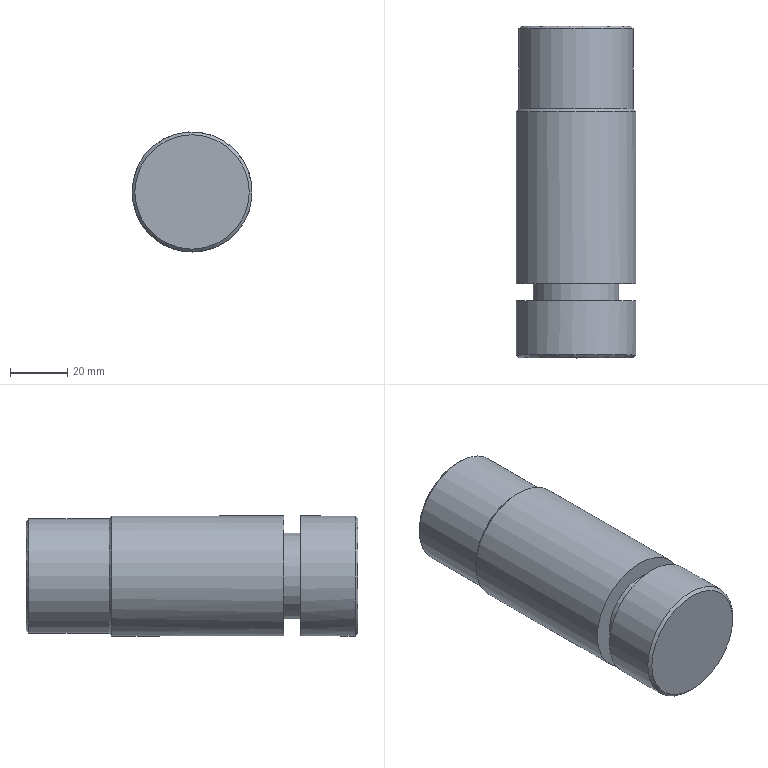Part | NX | features solid 2 | 1 solid | 11 faces | box 42 x 116 x 42 mm | volume 152713 mm3 | plane 4 | cylinder 4 | cone 3 | commonest cylinder face diameters 42 x2 30 x1 40 x1
STEP:
#1=CARTESIAN_POINT('',(-721.,-535.,180.));
#2=VERTEX_POINT('',#1);
#3=CARTESIAN_POINT('',(-700.,-535.,180.));
#4=DIRECTION('',(0.,1.,0.));
#5=DIRECTION('',(-1.,0.,0.));
#6=AXIS2_PLACEMENT_3D('',#3,#4,#5);
#7=CIRCLE('',#6,21.);
#8=EDGE_CURVE('',#2,#2,#7,.T.);
#9=ORIENTED_EDGE('',*,*,#8,.F.);
#10=EDGE_LOOP('',(#9));
#11=FACE_BOUND('',#10,.T.);
#12=CARTESIAN_POINT('',(-715.,-535.,180.));
#13=VERTEX_POINT('',#12);
#14=CARTESIAN_POINT('',(-700.,-535.,180.));
#15=DIRECTION('',(0.,1.,0.));
#16=DIRECTION('',(-1.,0.,0.));
#17=AXIS2_PLACEMENT_3D('',#14,#15,#16);
#18=CIRCLE('',#17,15.);
#19=EDGE_CURVE('',#13,#13,#18,.T.);
#20=ORIENTED_EDGE('',*,*,#19,.T.);
#21=EDGE_LOOP('',(#20));
#22=FACE_BOUND('',#21,.T.);
#23=CARTESIAN_POINT('',(-700.,-535.,180.));
#24=DIRECTION('',(0.,-1.,0.));
#25=DIRECTION('',(0.,0.,-1.));
#26=AXIS2_PLACEMENT_3D('',#23,#24,#25);
#27=PLANE('',#26);
#28=ADVANCED_FACE('',(#11,#22),#27,.T.);
#29=CARTESIAN_POINT('',(-721.,-475.,180.));
#30=VERTEX_POINT('',#29);
#31=CARTESIAN_POINT('',(-700.,-475.,180.));
#32=DIRECTION('',(0.,1.,0.));
#33=DIRECTION('',(-1.,0.,0.));
#34=AXIS2_PLACEMENT_3D('',#31,#32,#33);
#35=CIRCLE('',#34,21.);
#36=EDGE_CURVE('',#30,#30,#35,.T.);
#37=ORIENTED_EDGE('',*,*,#36,.F.);
#38=EDGE_LOOP('',(#37));
#39=FACE_BOUND('',#38,.T.);
#40=ORIENTED_EDGE('',*,*,#8,.T.);
#41=EDGE_LOOP('',(#40));
#42=FACE_BOUND('',#41,.T.);
#43=CARTESIAN_POINT('',(-700.,-535.,180.));
#44=DIRECTION('',(0.,1.,0.));
#45=DIRECTION('',(0.,0.,1.));
#46=AXIS2_PLACEMENT_3D('',#43,#44,#45);
#47=CYLINDRICAL_SURFACE('',#46,21.);
#48=ADVANCED_FACE('',(#39,#42),#47,.T.);
#49=CARTESIAN_POINT('',(-715.,-541.,180.));
#50=VERTEX_POINT('',#49);
#51=CARTESIAN_POINT('',(-700.,-541.,180.));
#52=DIRECTION('',(0.,1.,0.));
#53=DIRECTION('',(-1.,0.,0.));
#54=AXIS2_PLACEMENT_3D('',#51,#52,#53);
#55=CIRCLE('',#54,15.);
#56=EDGE_CURVE('',#50,#50,#55,.T.);
#57=ORIENTED_EDGE('',*,*,#56,.T.);
#58=EDGE_LOOP('',(#57));
#59=FACE_BOUND('',#58,.T.);
#60=ORIENTED_EDGE('',*,*,#19,.F.);
#61=EDGE_LOOP('',(#60));
#62=FACE_BOUND('',#61,.T.);
#63=CARTESIAN_POINT('',(-700.,-541.,180.));
#64=DIRECTION('',(0.,1.,0.));
#65=DIRECTION('',(0.,0.,1.));
#66=AXIS2_PLACEMENT_3D('',#63,#64,#65);
#67=CYLINDRICAL_SURFACE('',#66,15.);
#68=ADVANCED_FACE('',(#59,#62),#67,.T.);
#69=CARTESIAN_POINT('',(-721.,-541.,180.));
#70=VERTEX_POINT('',#69);
#71=CARTESIAN_POINT('',(-700.,-541.,180.));
#72=DIRECTION('',(0.,1.,0.));
#73=DIRECTION('',(-1.,0.,0.));
#74=AXIS2_PLACEMENT_3D('',#71,#72,#73);
#75=CIRCLE('',#74,21.);
#76=EDGE_CURVE('',#70,#70,#75,.T.);
#77=ORIENTED_EDGE('',*,*,#76,.T.);
#78=EDGE_LOOP('',(#77));
#79=FACE_BOUND('',#78,.T.);
#80=ORIENTED_EDGE('',*,*,#56,.F.);
#81=EDGE_LOOP('',(#80));
#82=FACE_BOUND('',#81,.T.);
#83=CARTESIAN_POINT('',(-700.,-541.,180.));
#84=DIRECTION('',(0.,-1.,0.));
#85=DIRECTION('',(0.,0.,-1.));
#86=AXIS2_PLACEMENT_3D('',#83,#84,#85);
#87=PLANE('',#86);
#88=ADVANCED_FACE('',(#79,#82),#87,.F.);
#89=ORIENTED_EDGE('',*,*,#76,.F.);
#90=EDGE_LOOP('',(#89));
#91=FACE_BOUND('',#90,.T.);
#92=CARTESIAN_POINT('',(-700.,-560.,159.));
#93=VERTEX_POINT('',#92);
#94=CARTESIAN_POINT('',(-700.,-560.,180.));
#95=DIRECTION('',(0.,1.,0.));
#96=DIRECTION('',(0.,0.,-1.));
#97=AXIS2_PLACEMENT_3D('',#94,#95,#96);
#98=CIRCLE('',#97,21.);
#99=EDGE_CURVE('',#93,#93,#98,.F.);
#100=ORIENTED_EDGE('',*,*,#99,.F.);
#101=EDGE_LOOP('',(#100));
#102=FACE_BOUND('',#101,.T.);
#103=CARTESIAN_POINT('',(-700.,-555.,180.));
#104=DIRECTION('',(0.,1.,0.));
#105=DIRECTION('',(0.,0.,1.));
#106=AXIS2_PLACEMENT_3D('',#103,#104,#105);
#107=CYLINDRICAL_SURFACE('',#106,21.);
#108=ADVANCED_FACE('',(#91,#102),#107,.T.);
#109=CARTESIAN_POINT('',(-700.,-561.,160.));
#110=VERTEX_POINT('',#109);
#111=CARTESIAN_POINT('',(-700.,-561.,180.));
#112=DIRECTION('',(0.,1.,0.));
#113=DIRECTION('',(0.,0.,-1.));
#114=AXIS2_PLACEMENT_3D('',#111,#112,#113);
#115=CIRCLE('',#114,20.);
#116=EDGE_CURVE('',#110,#110,#115,.T.);
#117=ORIENTED_EDGE('',*,*,#116,.F.);
#118=EDGE_LOOP('',(#117));
#119=FACE_BOUND('',#118,.T.);
#120=CARTESIAN_POINT('',(-700.,-561.,180.));
#121=DIRECTION('',(0.,-1.,0.));
#122=DIRECTION('',(0.,0.,-1.));
#123=AXIS2_PLACEMENT_3D('',#120,#121,#122);
#124=PLANE('',#123);
#125=ADVANCED_FACE('',(#119),#124,.T.);
#126=CARTESIAN_POINT('',(-700.,-474.,160.));
#127=VERTEX_POINT('',#126);
#128=CARTESIAN_POINT('',(-700.,-474.,180.));
#129=DIRECTION('',(0.,1.,0.));
#130=DIRECTION('',(0.,0.,-1.));
#131=AXIS2_PLACEMENT_3D('',#128,#129,#130);
#132=CIRCLE('',#131,20.);
#133=EDGE_CURVE('',#127,#127,#132,.F.);
#134=ORIENTED_EDGE('',*,*,#133,.F.);
#135=EDGE_LOOP('',(#134));
#136=FACE_BOUND('',#135,.T.);
#137=CARTESIAN_POINT('',(-700.,-446.,160.));
#138=VERTEX_POINT('',#137);
#139=CARTESIAN_POINT('',(-700.,-446.,180.));
#140=DIRECTION('',(0.,1.,0.));
#141=DIRECTION('',(0.,0.,-1.));
#142=AXIS2_PLACEMENT_3D('',#139,#140,#141);
#143=CIRCLE('',#142,20.);
#144=EDGE_CURVE('',#138,#138,#143,.T.);
#145=ORIENTED_EDGE('',*,*,#144,.F.);
#146=EDGE_LOOP('',(#145));
#147=FACE_BOUND('',#146,.T.);
#148=CARTESIAN_POINT('',(-700.,-405.,180.));
#149=DIRECTION('',(0.,-1.,0.));
#150=DIRECTION('',(0.,0.,-1.));
#151=AXIS2_PLACEMENT_3D('',#148,#149,#150);
#152=CYLINDRICAL_SURFACE('',#151,20.);
#153=ADVANCED_FACE('',(#136,#147),#152,.T.);
#154=CARTESIAN_POINT('',(-700.,-445.,161.));
#155=VERTEX_POINT('',#154);
#156=CARTESIAN_POINT('',(-700.,-445.,180.));
#157=DIRECTION('',(0.,1.,0.));
#158=DIRECTION('',(0.,0.,-1.));
#159=AXIS2_PLACEMENT_3D('',#156,#157,#158);
#160=CIRCLE('',#159,19.);
#161=EDGE_CURVE('',#155,#155,#160,.F.);
#162=ORIENTED_EDGE('',*,*,#161,.F.);
#163=EDGE_LOOP('',(#162));
#164=FACE_BOUND('',#163,.T.);
#165=CARTESIAN_POINT('',(-700.,-445.,180.));
#166=DIRECTION('',(0.,-1.,0.));
#167=DIRECTION('',(0.,0.,-1.));
#168=AXIS2_PLACEMENT_3D('',#165,#166,#167);
#169=PLANE('',#168);
#170=ADVANCED_FACE('',(#164),#169,.F.);
#171=ORIENTED_EDGE('',*,*,#161,.T.);
#172=EDGE_LOOP('',(#171));
#173=FACE_BOUND('',#172,.T.);
#174=ORIENTED_EDGE('',*,*,#144,.T.);
#175=EDGE_LOOP('',(#174));
#176=FACE_BOUND('',#175,.T.);
#177=CARTESIAN_POINT('',(-700.,-446.,180.));
#178=DIRECTION('',(0.,-1.,0.));
#179=DIRECTION('',(0.,0.,-1.));
#180=AXIS2_PLACEMENT_3D('',#177,#178,#179);
#181=CONICAL_SURFACE('',#180,20.,0.7854);
#182=ADVANCED_FACE('',(#173,#176),#181,.T.);
#183=ORIENTED_EDGE('',*,*,#133,.T.);
#184=EDGE_LOOP('',(#183));
#185=FACE_BOUND('',#184,.T.);
#186=ORIENTED_EDGE('',*,*,#36,.T.);
#187=EDGE_LOOP('',(#186));
#188=FACE_BOUND('',#187,.T.);
#189=CARTESIAN_POINT('',(-700.,-475.,180.));
#190=DIRECTION('',(0.,-1.,0.));
#191=DIRECTION('',(0.,0.,-1.));
#192=AXIS2_PLACEMENT_3D('',#189,#190,#191);
#193=CONICAL_SURFACE('',#192,21.,0.7854);
#194=ADVANCED_FACE('',(#185,#188),#193,.T.);
#195=ORIENTED_EDGE('',*,*,#99,.T.);
#196=EDGE_LOOP('',(#195));
#197=FACE_BOUND('',#196,.T.);
#198=ORIENTED_EDGE('',*,*,#116,.T.);
#199=EDGE_LOOP('',(#198));
#200=FACE_BOUND('',#199,.T.);
#201=CARTESIAN_POINT('',(-700.,-561.,180.));
#202=DIRECTION('',(0.,1.,0.));
#203=DIRECTION('',(0.,0.,1.));
#204=AXIS2_PLACEMENT_3D('',#201,#202,#203);
#205=CONICAL_SURFACE('',#204,20.,0.7854);
#206=ADVANCED_FACE('',(#197,#200),#205,.T.);
#207=CLOSED_SHELL('',(#28,#48,#68,#88,#108,#125,#153,#170,#182,#194,#206));
#208=MANIFOLD_SOLID_BREP('',#207);
#209=(LENGTH_UNIT()NAMED_UNIT(*)SI_UNIT(.MILLI.,.METRE.));
#210=UNCERTAINTY_MEASURE_WITH_UNIT(LENGTH_MEASURE(0.00001),#209,'','');
#211=(NAMED_UNIT(*)PLANE_ANGLE_UNIT()SI_UNIT($,.RADIAN.));
#212=(NAMED_UNIT(*)SI_UNIT($,.STERADIAN.)SOLID_ANGLE_UNIT());
#213=(GEOMETRIC_REPRESENTATION_CONTEXT(3)GLOBAL_UNCERTAINTY_ASSIGNED_CONTEXT((#210))GLOBAL_UNIT_ASSIGNED_CONTEXT((#209,#211,#212))REPRESENTATION_CONTEXT('',''));
#214=ADVANCED_BREP_SHAPE_REPRESENTATION('',(#208),#213);